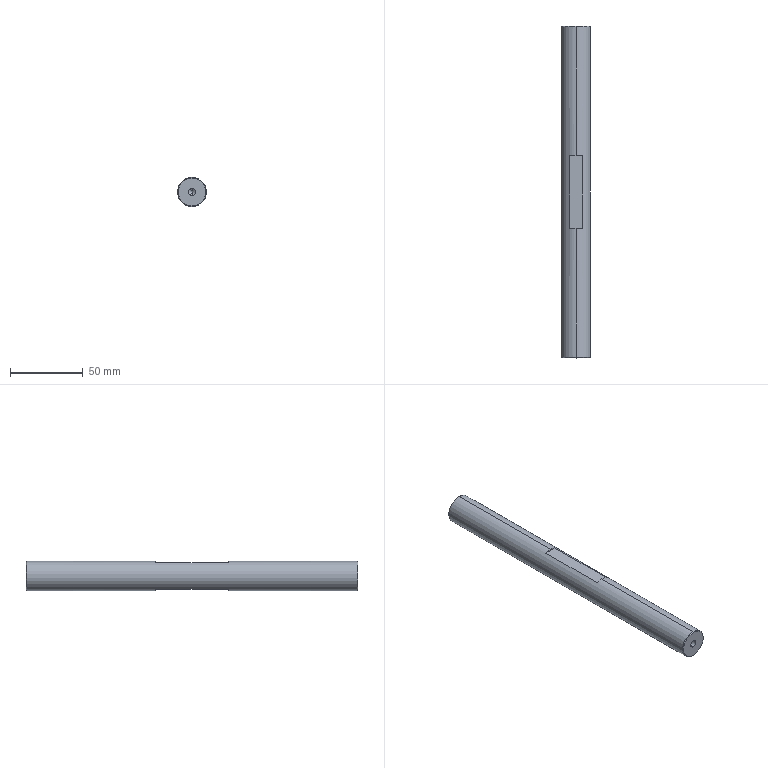Part | STEP file | PN_0007 | 1 solid | 25 faces | box 20 x 228 x 20 mm | volume 70235 mm3 | plane 9 | cone 8 | cylinder 8 | commonest cylinder face diameters 5 x4 6 x2 20 x2